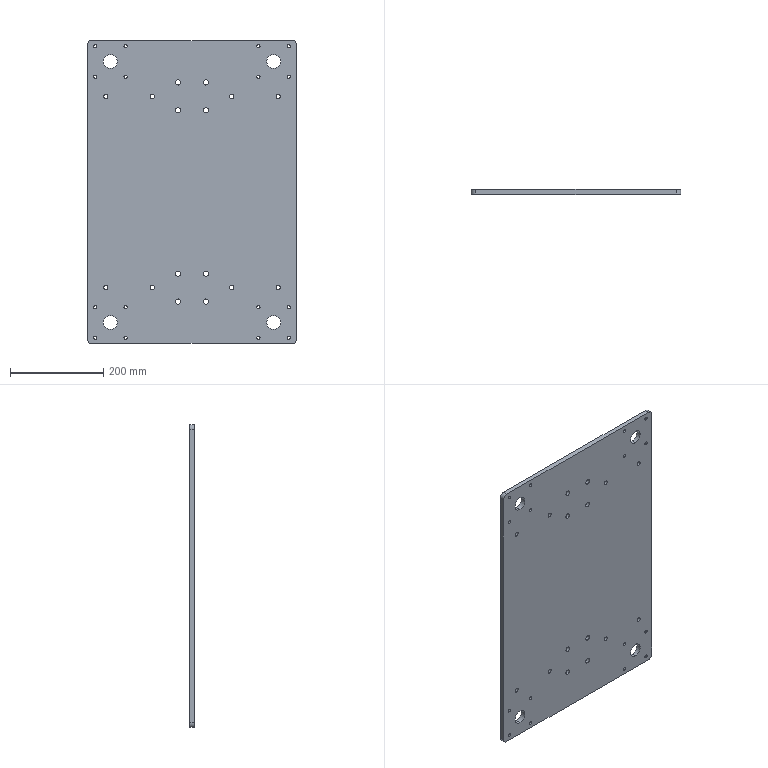Part | SolidWorks | features BaseBody 1 | 1 solid | 82 faces | box 450 x 10 x 650 mm | volume 2877018 mm3 | cylinder 76 | plane 6 | commonest cylinder face diameters 7 x32 9 x16 11 x16 30 x8 20 x4